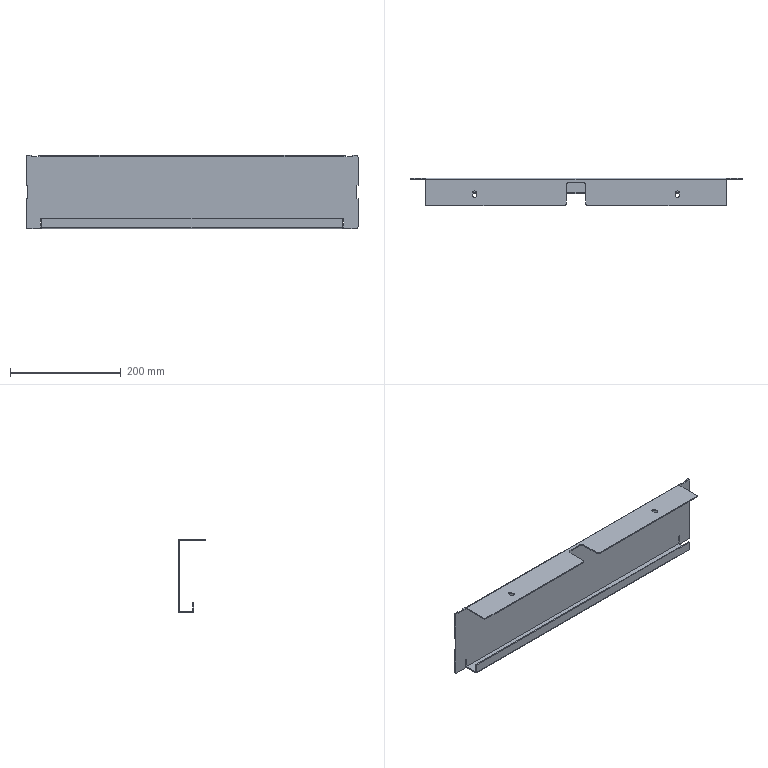Part | NX | features solid 2 | 1 solid | 77 faces | box 600 x 50 x 132 mm | volume 251124 mm3 | plane 62 | cylinder 15 | commonest cylinder face diameters 6 x4 7 x4 10 x4 4 x3